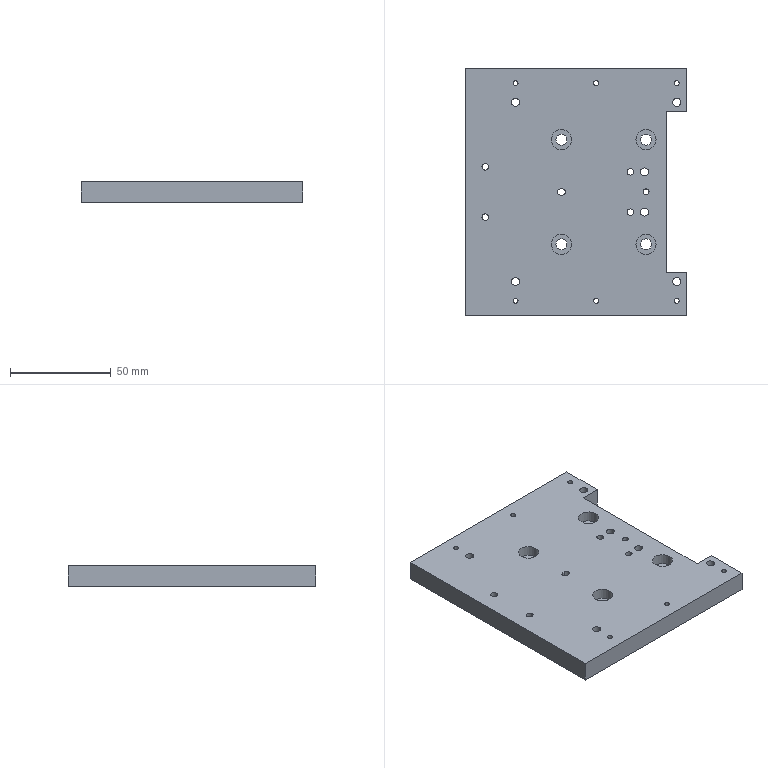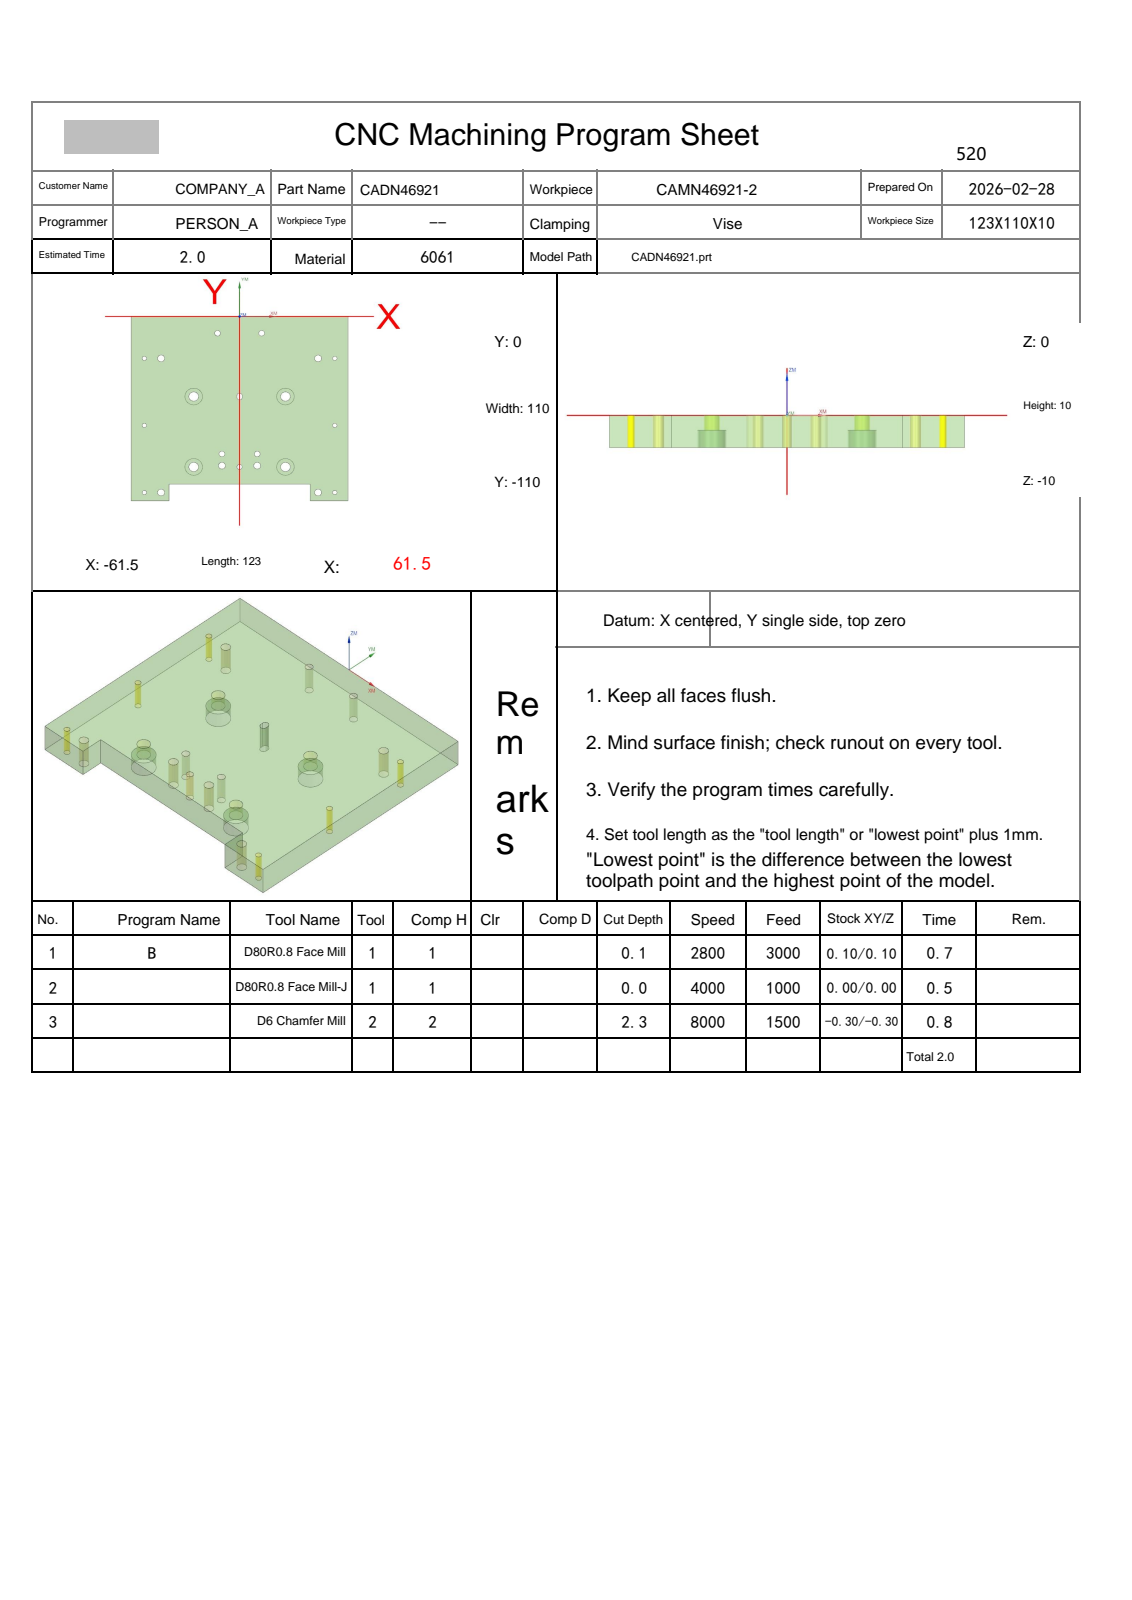NC program | NX | posted by the shop | part box 110 x 123 x 10 mm
Whole program:
%
O0001
(Machine time: 2.55 MIN)
(===Total Tool:2===)
(T1=D80R0.8 Face Mill D=80.  R=0.8  D-  H01 Z=0.    )
(T2=D6 Chamfer Mill   D=6.   R=0.   D-  H02 Z=-2.3  )
G80 G90 G17 G49 G40
G91 G28 Z0
M01
N1 T01 M06
(D80R0.8 Face Mill  D=80. R=0.8 H=01 ce=0.10 di=0.10)
G00 G90 G54 X113.597 Y-86.097 M03 S2800
G43 H01 Z50.
M08
Z3.525
G01 Z1.525 F3000.
X101.597
X-93.6
G02 X-101.597 Y-78.1 I.003 J8.
G01 Y-39.263
G02 X-93.597 Y-31.263 I8. J0.0
G01 X101.597
X113.597
Z3.525
G00 Y-86.097
Z3.05
G01 Z1.05
X101.597
X-93.6
G02 X-101.597 Y-78.1 I.003 J8.
G01 Y-39.263
G02 X-93.597 Y-31.263 I8. J0.0
G01 X101.597
X113.597
Z3.05
G00 Y-86.097
Z2.575
G01 Z.575
X101.597
X-93.6
G02 X-101.597 Y-78.1 I.003 J8.
G01 Y-39.263
G02 X-93.597 Y-31.263 I8. J0.0
G01 X101.597
X113.597
Z2.575
G00 Y-86.097
Z2.1
G01 Z.1
X101.597
X-93.6
G02 X-101.597 Y-78.1 I.003 J8.
G01 Y-39.263
G02 X-93.597 Y-31.263 I8. J0.0
G01 X101.597
X113.597
Z2.1
G00 Z50.
G91 G28 Z0.0
M05
M09
G91 G28 Z0.0
M01
N2 T01 M06
(D80R0.8 Face Mill-J  D=80. R=0.8 H=01 ce=0.00 di=0.00)
G00 G90 G54 X113.499 Y-85.999 M03 S4000
G43 H01 Z50.
M08
Z2.
G01 Z0.0 F1000.
X101.499
X-93.502
G02 X-101.499 Y-78.002 I.003 J8.
G01 Y-39.361
G02 X-93.499 Y-31.361 I8. J0.0
G01 X101.499
X113.499
Z2.
G00 Z50.
G91 G28 Z0.0
M05
M09
G91 G28 Z0.0
M01
N3 T02 M06
(D6 Chamfer Mill  D=6. R=0. H=02 ce=0.00 di=0.00)
G00 G90 G54 X-54. Y-105. M03 S8000
G43 H02 Z50.
M08
G98 G81 X-54. Y-105. Z-1.75 R3. F1000.
Y-65.
Y-25.
X54.
Y-65.
Y-105.
G80
G00 Z50.
G00 G90 X0.0 Y-89.75 M03 S8000
Z50.
G98 G81 X0.0 Y-89.75 Z-1.8 R3. F1000.
G80
G00 Z50.
G00 G90 X44.5 Y-25. M03 S8000
Z50.
G98 G81 X44.5 Y-25. Z-2.3 R3. F1000.
Y-105.
X10. Y-89.
X-10.
X-44.5 Y-105.
Y-25.
G80
G00 Z50.
G00 G90 X12.5 Y-10. M03 S8000
Z50.
G98 G81 X12.5 Y-10. Z-2.2 R3. F1000.
X-12.5
X-10. Y-82.
X10.
G80
G00 Z50.
G00 G90 X-25.353 Y-89.685 M03 S8000
Z50.
Z-.9
G01 Z-1.4 F1200.
X-24.5 Y-89.6
G03 X-26. Y-88.1 I-1.5 J0.0
X-27.65 Y-89.75 I0.0 J-1.65
X-26. Y-91.4 I1.65 J0.0
X-24.35 Y-89.75 I0.0 J1.65
X-26. Y-88.1 I-1.65 J0.0
X-27.5 Y-89.6 I0.0 J-1.5
G01 X-26.647 Y-89.685
Z-.9
G00 Z50.
X-25.353 Y-47.685
Z-.9
G01 Z-1.4
X-24.5 Y-47.6
G03 X-26. Y-46.1 I-1.5 J0.0
X-27.65 Y-47.75 I0.0 J-1.65
X-26. Y-49.4 I1.65 J0.0
X-24.35 Y-47.75 I0.0 J1.65
X-26. Y-46.1 I-1.65 J0.0
X-27.5 Y-47.6 I0.0 J-1.5
G01 X-26.647 Y-47.685
Z-.9
G00 Z50.
X26.647
Z-.9
G01 Z-1.4
X27.5 Y-47.6
G03 X26. Y-46.1 I-1.5 J0.0
X24.35 Y-47.75 I0.0 J-1.65
X26. Y-49.4 I1.65 J0.0
X27.65 Y-47.75 I0.0 J1.65
X26. Y-46.1 I-1.65 J0.0
X24.5 Y-47.6 I0.0 J-1.5
G01 X25.353 Y-47.685
Z-.9
G00 Z50.
X26.647 Y-89.685
Z-.9
G01 Z-1.4
X27.5 Y-89.6
G03 X26. Y-88.1 I-1.5 J0.0
X24.35 Y-89.75 I0.0 J-1.65
X26. Y-91.4 I1.65 J0.0
X27.65 Y-89.75 I0.0 J1.65
X26. Y-88.1 I-1.65 J0.0
X24.5 Y-89.6 I0.0 J-1.5
G01 X25.353 Y-89.685
Z-.9
G00 Z50.
G00 G90 X-.386 Y1.227 M03 S6500
Z50.
Z.172
G01 Z-1.2 F1500.
G03 X-.1 Y1.027 I1.286 J1.532
G01 X-.054 Y.997
X0.0 Y1.
X61.5
G02 X62.5 Y0.0 I0.0 J-1.
G01 Y-110.
G02 X61.5 Y-111. I-1. J0.0
G01 X40.
G02 X39. Y-110. I0.0 J1.
G01 Y-101.
X-39.
Y-110.
G02 X-40. Y-111. I-1. J0.0
G01 X-61.5
G02 X-62.5 Y-110. I0.0 J1.
G01 Y0.0
G02 X-61.5 Y1. I1. J0.0
G01 X0.0
X.054 Y.997
X.1 Y1.027
G03 X.386 Y1.227 I-1. J1.732
G01 Z.172
G00 Z10.
X44.912 Y-104.174
Z.33
G01 Z-1.2
G03 X44.603 Y-104.014 I-1.075 J-1.687
G01 X44.554 Y-103.99
X44.5 Y-104.
G03 X43.5 Y-105. I0.0 J-1.
X44.5 Y-106. I1. J0.0
X45.5 Y-105. I0.0 J1.
X44.5 Y-104. I-1. J0.0
G01 X44.446 Y-103.99
X44.397 Y-104.014
G03 X44.088 Y-104.174 I.765 J-1.848
G01 Z.33
G00 Z10.
X26.407 Y-88.185
Z.27
G01 Z-1.2
G03 X26.102 Y-88.016 I-1.118 J-1.658
G01 X26.054 Y-87.991
X26. Y-88.
G03 X24.25 Y-89.75 I0.0 J-1.75
X26. Y-91.5 I1.75 J0.0
X27.75 Y-89.75 I0.0 J1.75
X26. Y-88. I-1.75 J0.0
G01 X25.946 Y-87.991
X25.898 Y-88.016
G03 X25.593 Y-88.185 I.813 J-1.827
G01 Z.27
G00 Z10.
X10.419 Y-81.506
Z.405
G01 Z-1.2
G03 X10.103 Y-81.359 I-1. J-1.732
G01 X10.053 Y-81.338
X10. Y-81.35
G03 X9.35 Y-82. I0.0 J-.65
X10. Y-82.65 I.65 J0.0
X10.65 Y-82. I0.0 J.65
X10. Y-81.35 I-.65 J0.0
G01 X9.947 Y-81.338
X9.897 Y-81.359
G03 X9.581 Y-81.506 I.684 J-1.879
G01 Z.405
G00 Z2.55
X10.412 Y-88.174
Z.33
G01 Z-1.2
G03 X10.103 Y-88.014 I-1.075 J-1.687
G01 X10.054 Y-87.99
X10. Y-88.
G03 X9. Y-89. I0.0 J-1.
X10. Y-90. I1. J0.0
X11. Y-89. I0.0 J1.
X10. Y-88. I-1. J0.0
G01 X9.946 Y-87.99
X9.897 Y-88.014
G03 X9.588 Y-88.174 I.765 J-1.848
G01 Z.33
G00 Z2.55
X.419 Y-89.406
Z.447
G01 Z-1.2
G03 X.103 Y-89.259 I-1. J-1.732
G01 X.053 Y-89.238
X0.0 Y-89.25
G03 X-.5 Y-89.75 I0.0 J-.5
X0.0 Y-90.25 I.5 J0.0
X.5 Y-89.75 I0.0 J.5
X0.0 Y-89.25 I-.5 J0.0
G01 X-.053 Y-89.238
X-.103 Y-89.259
G03 X-.419 Y-89.406 I.684 J-1.879
G01 Z.447
G00 Z2.55
X-9.588 Y-88.174
Z.33
G01 Z-1.2
G03 X-9.897 Y-88.014 I-1.075 J-1.687
G01 X-9.946 Y-87.99
X-10. Y-88.
G03 X-11. Y-89. I0.0 J-1.
X-10. Y-90. I1. J0.0
X-9. Y-89. I0.0 J1.
X-10. Y-88. I-1. J0.0
G01 X-10.054 Y-87.99
X-10.103 Y-88.014
G03 X-10.412 Y-88.174 I.765 J-1.848
G01 Z.33
G00 Z2.55
X-9.581 Y-81.506
Z.405
G01 Z-1.2
G03 X-9.897 Y-81.359 I-1. J-1.732
G01 X-9.947 Y-81.338
X-10. Y-81.35
G03 X-10.65 Y-82. I0.0 J-.65
X-10. Y-82.65 I.65 J0.0
X-9.35 Y-82. I0.0 J.65
X-10. Y-81.35 I-.65 J0.0
G01 X-10.053 Y-81.338
X-10.103 Y-81.359
G03 X-10.419 Y-81.506 I.684 J-1.879
G01 Z.405
G00 Z10.
X-25.593 Y-88.185
Z.27
G01 Z-1.2
G03 X-25.898 Y-88.016 I-1.118 J-1.658
G01 X-25.946 Y-87.991
X-26. Y-88.
G03 X-27.75 Y-89.75 I0.0 J-1.75
X-26. Y-91.5 I1.75 J0.0
X-24.25 Y-89.75 I0.0 J1.75
X-26. Y-88. I-1.75 J0.0
G01 X-26.054 Y-87.991
X-26.102 Y-88.016
G03 X-26.407 Y-88.185 I.813 J-1.827
G01 Z.27
G00 Z10.
X-44.088 Y-104.174
Z.33
G01 Z-1.2
G03 X-44.397 Y-104.014 I-1.075 J-1.687
G01 X-44.446 Y-103.99
X-44.5 Y-104.
G03 X-45.5 Y-105. I0.0 J-1.
X-44.5 Y-106. I1. J0.0
X-43.5 Y-105. I0.0 J1.
X-44.5 Y-104. I-1. J0.0
G01 X-44.554 Y-103.99
X-44.603 Y-104.014
G03 X-44.912 Y-104.174 I.765 J-1.848
G01 Z.33
G00 Z10.
X-25.593 Y-46.185
Z.27
G01 Z-1.2
G03 X-25.898 Y-46.016 I-1.118 J-1.658
G01 X-25.946 Y-45.991
X-26. Y-46.
G03 X-27.75 Y-47.75 I0.0 J-1.75
X-26. Y-49.5 I1.75 J0.0
X-24.25 Y-47.75 I0.0 J1.75
X-26. Y-46. I-1.75 J0.0
G01 X-26.054 Y-45.991
X-26.102 Y-46.016
G03 X-26.407 Y-46.185 I.813 J-1.827
G01 Z.27
G00 Z10.
X.273 Y-48.136
Z.172
G01 Z-1.2
G03 X.473 Y-47.85 I-1.532 J1.286
G01 X.503 Y-47.804
X.5 Y-47.75
Y-47.25
G03 X0.0 Y-46.75 I-.5 J0.0
G01 X-.191 Y-46.788
X-.354 Y-46.896
X-.462 Y-47.059
X-.5 Y-47.25
Y-48.25
G03 X0.0 Y-48.75 I.5 J0.0
G01 X.191 Y-48.712
X.354 Y-48.604
X.462 Y-48.441
X.5 Y-48.25
Y-47.75
X.503 Y-47.696
X.473 Y-47.65
G03 X.273 Y-47.364 I-1.732 J-1.
G01 Z.172
G00 Z10.
X26.407 Y-46.185
Z.27
G01 Z-1.2
G03 X26.102 Y-46.016 I-1.118 J-1.658
G01 X26.054 Y-45.991
X26. Y-46.
G03 X24.25 Y-47.75 I0.0 J-1.75
X26. Y-49.5 I1.75 J0.0
X27.75 Y-47.75 I0.0 J1.75
X26. Y-46. I-1.75 J0.0
G01 X25.946 Y-45.991
X25.898 Y-46.016
G03 X25.593 Y-46.185 I.813 J-1.827
G01 Z.27
G00 Z10.
X44.912 Y-24.174
Z.33
G01 Z-1.2
G03 X44.603 Y-24.014 I-1.075 J-1.687
G01 X44.554 Y-23.99
X44.5 Y-24.
G03 X43.5 Y-25. I0.0 J-1.
X44.5 Y-26. I1. J0.0
X45.5 Y-25. I0.0 J1.
X44.5 Y-24. I-1. J0.0
G01 X44.446 Y-23.99
X44.397 Y-24.014
G03 X44.088 Y-24.174 I.765 J-1.848
G01 Z.33
G00 Z10.
X12.919 Y-9.506
Z.405
G01 Z-1.2
G03 X12.603 Y-9.359 I-1. J-1.732
G01 X12.553 Y-9.338
X12.5 Y-9.35
G03 X11.85 Y-10. I0.0 J-.65
X12.5 Y-10.65 I.65 J0.0
X13.15 Y-10. I0.0 J.65
X12.5 Y-9.35 I-.65 J0.0
G01 X12.447 Y-9.338
X12.397 Y-9.359
G03 X12.081 Y-9.506 I.684 J-1.879
G01 Z.405
G00 Z10.
X-12.081
Z.405
G01 Z-1.2
G03 X-12.397 Y-9.359 I-1. J-1.732
G01 X-12.447 Y-9.338
X-12.5 Y-9.35
G03 X-13.15 Y-10. I0.0 J-.65
X-12.5 Y-10.65 I.65 J0.0
X-11.85 Y-10. I0.0 J.65
X-12.5 Y-9.35 I-.65 J0.0
G01 X-12.553 Y-9.338
X-12.603 Y-9.359
G03 X-12.919 Y-9.506 I.684 J-1.879
G01 Z.405
G00 Z10.
X-44.088 Y-24.174
Z.33
G01 Z-1.2
G03 X-44.397 Y-24.014 I-1.075 J-1.687
G01 X-44.446 Y-23.99
X-44.5 Y-24.
G03 X-45.5 Y-25. I0.0 J-1.
X-44.5 Y-26. I1. J0.0
X-43.5 Y-25. I0.0 J1.
X-44.5 Y-24. I-1. J0.0
G01 X-44.554 Y-23.99
X-44.603 Y-24.014
G03 X-44.912 Y-24.174 I.765 J-1.848
G01 Z.33
G00 Z50.
M05
M09
G91 G28 Z0.0
G91 G28 Y0.0
M30
%